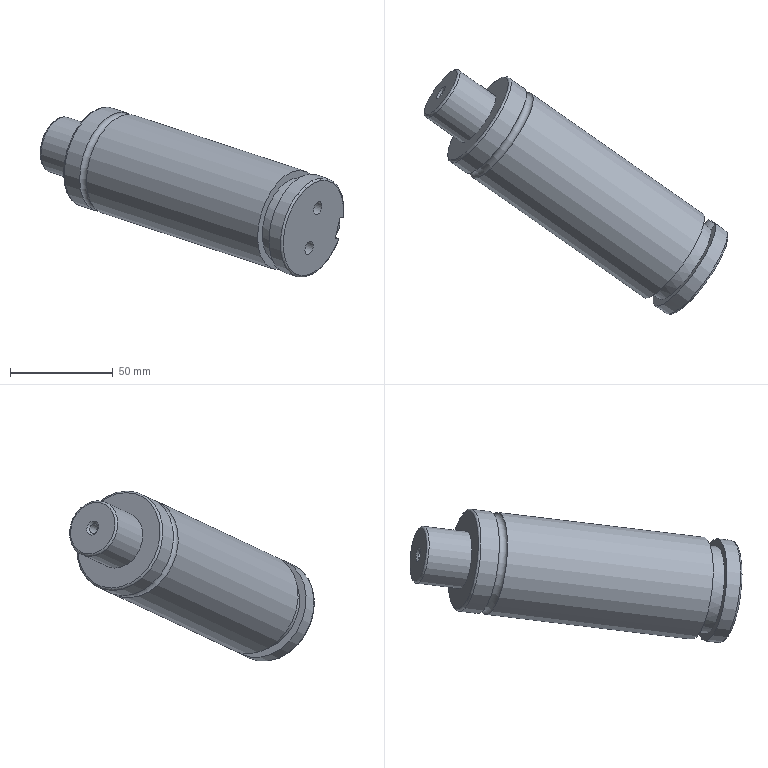Part | NX | features 1 2 | 1 solid | 34 faces | box 148.12 x 119.315 x 82.981 mm | volume 275318 mm3 | plane 16 | cylinder 10 | torus 4 | cone 4 | commonest cylinder face diameters 50.2 x3 6.6 x2 4.9 x1 9.5 x1 11 x1 28 x1
STEP:
#1=CARTESIAN_POINT('',(-931.05,560.37,-211.525));
#2=VERTEX_POINT('',#1);
#3=CARTESIAN_POINT('',(-936.371,564.096,-235.77));
#4=DIRECTION('',(-0.7912,0.554,0.2588));
#5=DIRECTION('',(0.212,-0.1485,0.9659));
#6=AXIS2_PLACEMENT_3D('',#3,#4,#5);
#7=CIRCLE('',#6,25.1);
#8=EDGE_CURVE('',#2,#2,#7,.T.);
#9=ORIENTED_EDGE('',*,*,#8,.T.);
#10=EDGE_LOOP('',(#9));
#11=FACE_BOUND('',#10,.T.);
#12=CARTESIAN_POINT('',(-934.373,562.697,-210.438));
#13=VERTEX_POINT('',#12);
#14=CARTESIAN_POINT('',(-939.694,566.423,-234.683));
#15=DIRECTION('',(-0.7912,0.554,0.2588));
#16=DIRECTION('',(0.212,-0.1485,0.9659));
#17=AXIS2_PLACEMENT_3D('',#14,#15,#16);
#18=CIRCLE('',#17,25.1);
#19=EDGE_CURVE('',#13,#13,#18,.T.);
#20=ORIENTED_EDGE('',*,*,#19,.F.);
#21=EDGE_LOOP('',(#20));
#22=FACE_BOUND('',#21,.T.);
#23=CARTESIAN_POINT('',(-938.033,565.259,-235.227));
#24=DIRECTION('',(-0.7912,0.554,0.2588));
#25=DIRECTION('',(-0.5736,-0.8192,0.));
#26=AXIS2_PLACEMENT_3D('',#23,#24,#25);
#27=TOROIDAL_SURFACE('',#26,25.1,2.1);
#28=ADVANCED_FACE('',(#11,#22),#27,.F.);
#29=CARTESIAN_POINT('',(-941.81,567.905,-208.005));
#30=VERTEX_POINT('',#29);
#31=CARTESIAN_POINT('',(-947.132,571.631,-232.25));
#32=DIRECTION('',(-0.7912,0.554,0.2588));
#33=DIRECTION('',(0.212,-0.1485,0.9659));
#34=AXIS2_PLACEMENT_3D('',#31,#32,#33);
#35=CIRCLE('',#34,25.1);
#36=EDGE_CURVE('',#30,#30,#35,.T.);
#37=ORIENTED_EDGE('',*,*,#36,.T.);
#38=EDGE_LOOP('',(#37));
#39=FACE_BOUND('',#38,.T.);
#40=CARTESIAN_POINT('',(-942.814,568.607,-208.713));
#41=VERTEX_POINT('',#40);
#42=CARTESIAN_POINT('',(-947.923,572.185,-231.991));
#43=DIRECTION('',(-0.7912,0.554,0.2588));
#44=DIRECTION('',(0.212,-0.1485,0.9659));
#45=AXIS2_PLACEMENT_3D('',#42,#43,#44);
#46=CIRCLE('',#45,24.1);
#47=EDGE_CURVE('',#41,#41,#46,.T.);
#48=ORIENTED_EDGE('',*,*,#47,.F.);
#49=EDGE_LOOP('',(#48));
#50=FACE_BOUND('',#49,.T.);
#51=CARTESIAN_POINT('',(-947.132,571.631,-232.25));
#52=DIRECTION('',(-0.7912,0.554,0.2588));
#53=DIRECTION('',(-0.5736,-0.8192,0.));
#54=AXIS2_PLACEMENT_3D('',#51,#52,#53);
#55=TOROIDAL_SURFACE('',#54,24.1,1.);
#56=ADVANCED_FACE('',(#39,#50),#55,.T.);
#57=ORIENTED_EDGE('',*,*,#19,.T.);
#58=EDGE_LOOP('',(#57));
#59=FACE_BOUND('',#58,.T.);
#60=ORIENTED_EDGE('',*,*,#36,.F.);
#61=EDGE_LOOP('',(#60));
#62=FACE_BOUND('',#61,.T.);
#63=CARTESIAN_POINT('',(-943.413,569.027,-233.467));
#64=DIRECTION('',(0.7912,-0.554,-0.2588));
#65=DIRECTION('',(0.5736,0.8192,0.));
#66=AXIS2_PLACEMENT_3D('',#63,#64,#65);
#67=CYLINDRICAL_SURFACE('',#66,25.1);
#68=ADVANCED_FACE('',(#59,#62),#67,.T.);
#69=CARTESIAN_POINT('',(-847.653,501.975,-238.805));
#70=VERTEX_POINT('',#69);
#71=CARTESIAN_POINT('',(-852.974,505.701,-263.05));
#72=DIRECTION('',(-0.7912,0.554,0.2588));
#73=DIRECTION('',(0.212,-0.1485,0.9659));
#74=AXIS2_PLACEMENT_3D('',#71,#72,#73);
#75=CIRCLE('',#74,25.1);
#76=EDGE_CURVE('',#70,#70,#75,.T.);
#77=ORIENTED_EDGE('',*,*,#76,.T.);
#78=EDGE_LOOP('',(#77));
#79=FACE_BOUND('',#78,.T.);
#80=ORIENTED_EDGE('',*,*,#8,.F.);
#81=EDGE_LOOP('',(#80));
#82=FACE_BOUND('',#81,.T.);
#83=CARTESIAN_POINT('',(-889.134,531.02,-251.222));
#84=DIRECTION('',(0.7912,-0.554,-0.2588));
#85=DIRECTION('',(0.5736,0.8192,0.));
#86=AXIS2_PLACEMENT_3D('',#83,#84,#85);
#87=CYLINDRICAL_SURFACE('',#86,25.1);
#88=ADVANCED_FACE('',(#79,#82),#87,.T.);
#89=CARTESIAN_POINT('',(-848.459,502.539,-242.475));
#90=VERTEX_POINT('',#89);
#91=CARTESIAN_POINT('',(-852.974,505.701,-263.05));
#92=DIRECTION('',(-0.7912,0.554,0.2588));
#93=DIRECTION('',(0.212,-0.1485,0.9659));
#94=AXIS2_PLACEMENT_3D('',#91,#92,#93);
#95=CIRCLE('',#94,21.3);
#96=EDGE_CURVE('',#90,#90,#95,.T.);
#97=ORIENTED_EDGE('',*,*,#96,.F.);
#98=EDGE_LOOP('',(#97));
#99=FACE_BOUND('',#98,.T.);
#100=CARTESIAN_POINT('',(-836.663,519.519,-269.81));
#101=VERTEX_POINT('',#100);
#102=CARTESIAN_POINT('',(-834.491,517.998,-259.913));
#103=VERTEX_POINT('',#102);
#104=CARTESIAN_POINT('',(-847.436,501.823,-264.861));
#105=DIRECTION('',(-0.7912,0.554,0.2588));
#106=DIRECTION('',(0.212,-0.1485,0.9659));
#107=AXIS2_PLACEMENT_3D('',#104,#105,#106);
#108=CIRCLE('',#107,21.3);
#109=EDGE_CURVE('',#101,#103,#108,.T.);
#110=ORIENTED_EDGE('',*,*,#109,.T.);
#111=CARTESIAN_POINT('',(-834.491,517.998,-259.913));
#112=CARTESIAN_POINT('',(-835.338,518.713,-260.035));
#113=CARTESIAN_POINT('',(-836.848,520.175,-260.94));
#114=CARTESIAN_POINT('',(-838.206,521.481,-263.862));
#115=CARTESIAN_POINT('',(-838.253,521.159,-267.327));
#116=CARTESIAN_POINT('',(-837.339,520.114,-269.153));
#117=CARTESIAN_POINT('',(-836.663,519.519,-269.81));
#118=B_SPLINE_CURVE_WITH_KNOTS('',3,(#111,#112,#113,#114,#115,#116,#117),.UNSPECIFIED.,.F.,.F.,(4,1,1,1,4),(0.,0.003296,0.006593,0.009889,0.01319),.UNSPECIFIED.);
#119=EDGE_CURVE('',#103,#101,#118,.T.);
#120=ORIENTED_EDGE('',*,*,#119,.T.);
#121=EDGE_LOOP('',(#110,#120));
#122=FACE_BOUND('',#121,.T.);
#123=CARTESIAN_POINT('',(-850.205,503.762,-263.956));
#124=DIRECTION('',(0.7912,-0.554,-0.2588));
#125=DIRECTION('',(0.5736,0.8192,0.));
#126=AXIS2_PLACEMENT_3D('',#123,#124,#125);
#127=CYLINDRICAL_SURFACE('',#126,21.3);
#128=ADVANCED_FACE('',(#99,#122),#127,.T.);
#129=CARTESIAN_POINT('',(-962.362,582.295,-212.774));
#130=VERTEX_POINT('',#129);
#131=CARTESIAN_POINT('',(-965.331,584.374,-226.297));
#132=DIRECTION('',(-0.7912,0.554,0.2588));
#133=DIRECTION('',(0.212,-0.1485,0.9659));
#134=AXIS2_PLACEMENT_3D('',#131,#132,#133);
#135=CIRCLE('',#134,14.);
#136=EDGE_CURVE('',#130,#130,#135,.T.);
#137=ORIENTED_EDGE('',*,*,#136,.T.);
#138=EDGE_LOOP('',(#137));
#139=FACE_BOUND('',#138,.T.);
#140=CARTESIAN_POINT('',(-963.366,582.998,-213.482));
#141=VERTEX_POINT('',#140);
#142=CARTESIAN_POINT('',(-966.122,584.928,-226.039));
#143=DIRECTION('',(-0.7912,0.554,0.2588));
#144=DIRECTION('',(0.212,-0.1485,0.9659));
#145=AXIS2_PLACEMENT_3D('',#142,#143,#144);
#146=CIRCLE('',#145,13.);
#147=EDGE_CURVE('',#141,#141,#146,.T.);
#148=ORIENTED_EDGE('',*,*,#147,.F.);
#149=EDGE_LOOP('',(#148));
#150=FACE_BOUND('',#149,.T.);
#151=CARTESIAN_POINT('',(-965.331,584.374,-226.297));
#152=DIRECTION('',(-0.7912,0.554,0.2588));
#153=DIRECTION('',(-0.5736,-0.8192,0.));
#154=AXIS2_PLACEMENT_3D('',#151,#152,#153);
#155=TOROIDAL_SURFACE('',#154,13.,1.);
#156=ADVANCED_FACE('',(#139,#150),#155,.T.);
#157=CARTESIAN_POINT('',(-944.955,570.107,-218.468));
#158=VERTEX_POINT('',#157);
#159=CARTESIAN_POINT('',(-947.923,572.185,-231.991));
#160=DIRECTION('',(0.7912,-0.554,-0.2588));
#161=DIRECTION('',(0.212,-0.1485,0.9659));
#162=AXIS2_PLACEMENT_3D('',#159,#160,#161);
#163=CIRCLE('',#162,14.);
#164=EDGE_CURVE('',#158,#158,#163,.T.);
#165=ORIENTED_EDGE('',*,*,#164,.F.);
#166=EDGE_LOOP('',(#165));
#167=FACE_BOUND('',#166,.T.);
#168=ORIENTED_EDGE('',*,*,#136,.F.);
#169=EDGE_LOOP('',(#168));
#170=FACE_BOUND('',#169,.T.);
#171=CARTESIAN_POINT('',(-956.627,578.279,-229.144));
#172=DIRECTION('',(0.7912,-0.554,-0.2588));
#173=DIRECTION('',(0.5736,0.8192,0.));
#174=AXIS2_PLACEMENT_3D('',#171,#172,#173);
#175=CYLINDRICAL_SURFACE('',#174,14.);
#176=ADVANCED_FACE('',(#167,#170),#175,.T.);
#177=CARTESIAN_POINT('',(-839.685,496.396,-260.46));
#178=VERTEX_POINT('',#177);
#179=CARTESIAN_POINT('',(-838.986,495.906,-257.273));
#180=DIRECTION('',(-0.7912,0.554,0.2588));
#181=DIRECTION('',(-0.212,0.1485,-0.9659));
#182=AXIS2_PLACEMENT_3D('',#179,#180,#181);
#183=CIRCLE('',#182,3.3);
#184=EDGE_CURVE('',#178,#178,#183,.T.);
#185=ORIENTED_EDGE('',*,*,#184,.F.);
#186=EDGE_LOOP('',(#185));
#187=FACE_BOUND('',#186,.T.);
#188=CARTESIAN_POINT('',(-848.547,502.601,-257.561));
#189=VERTEX_POINT('',#188);
#190=CARTESIAN_POINT('',(-847.848,502.111,-254.374));
#191=DIRECTION('',(0.7912,-0.554,-0.2588));
#192=DIRECTION('',(-0.212,0.1485,-0.9659));
#193=AXIS2_PLACEMENT_3D('',#190,#191,#192);
#194=CIRCLE('',#193,3.3);
#195=EDGE_CURVE('',#189,#189,#194,.T.);
#196=ORIENTED_EDGE('',*,*,#195,.F.);
#197=EDGE_LOOP('',(#196));
#198=FACE_BOUND('',#197,.T.);
#199=CARTESIAN_POINT('',(-843.417,499.009,-255.823));
#200=DIRECTION('',(-0.7912,0.554,0.2588));
#201=DIRECTION('',(-0.5736,-0.8192,0.));
#202=AXIS2_PLACEMENT_3D('',#199,#200,#201);
#203=CYLINDRICAL_SURFACE('',#202,3.3);
#204=ADVANCED_FACE('',(#187,#198),#203,.F.);
#205=ORIENTED_EDGE('',*,*,#195,.T.);
#206=EDGE_LOOP('',(#205));
#207=FACE_BOUND('',#206,.T.);
#208=CARTESIAN_POINT('',(-845.711,500.615,-255.073));
#209=VERTEX_POINT('',#208);
#210=VERTEX_LOOP('',#209);
#211=FACE_BOUND('',#210,.T.);
#212=CARTESIAN_POINT('',(-846.779,501.363,-254.723));
#213=DIRECTION('',(-0.7912,0.554,0.2588));
#214=DIRECTION('',(-0.5736,-0.8192,0.));
#215=AXIS2_PLACEMENT_3D('',#212,#213,#214);
#216=CONICAL_SURFACE('',#215,1.65,0.8851);
#217=ADVANCED_FACE('',(#207,#211),#216,.T.);
#218=CARTESIAN_POINT('',(-965.38,584.408,-222.658));
#219=VERTEX_POINT('',#218);
#220=CARTESIAN_POINT('',(-966.122,584.928,-226.039));
#221=DIRECTION('',(0.7912,-0.554,-0.2588));
#222=DIRECTION('',(0.212,-0.1485,0.9659));
#223=AXIS2_PLACEMENT_3D('',#220,#221,#222);
#224=CIRCLE('',#223,3.5);
#225=EDGE_CURVE('',#219,#219,#224,.T.);
#226=ORIENTED_EDGE('',*,*,#225,.F.);
#227=EDGE_LOOP('',(#226));
#228=FACE_BOUND('',#227,.T.);
#229=CARTESIAN_POINT('',(-964.772,583.982,-223.944));
#230=VERTEX_POINT('',#229);
#231=CARTESIAN_POINT('',(-965.291,584.346,-226.31));
#232=DIRECTION('',(-0.7912,0.554,0.2588));
#233=DIRECTION('',(0.212,-0.1485,0.9659));
#234=AXIS2_PLACEMENT_3D('',#231,#232,#233);
#235=CIRCLE('',#234,2.45);
#236=EDGE_CURVE('',#230,#230,#235,.T.);
#237=ORIENTED_EDGE('',*,*,#236,.F.);
#238=EDGE_LOOP('',(#237));
#239=FACE_BOUND('',#238,.T.);
#240=CARTESIAN_POINT('',(-965.706,584.637,-226.174));
#241=DIRECTION('',(-0.7912,0.554,0.2588));
#242=DIRECTION('',(-0.5736,-0.8192,0.));
#243=AXIS2_PLACEMENT_3D('',#240,#241,#242);
#244=CONICAL_SURFACE('',#243,2.975,0.7854);
#245=ADVANCED_FACE('',(#228,#239),#244,.F.);
#246=ORIENTED_EDGE('',*,*,#236,.T.);
#247=EDGE_LOOP('',(#246));
#248=FACE_BOUND('',#247,.T.);
#249=CARTESIAN_POINT('',(-960.459,580.963,-225.354));
#250=VERTEX_POINT('',#249);
#251=CARTESIAN_POINT('',(-960.979,581.326,-227.721));
#252=DIRECTION('',(-0.7912,0.554,0.2588));
#253=DIRECTION('',(0.212,-0.1485,0.9659));
#254=AXIS2_PLACEMENT_3D('',#251,#252,#253);
#255=CIRCLE('',#254,2.45);
#256=EDGE_CURVE('',#250,#250,#255,.T.);
#257=ORIENTED_EDGE('',*,*,#256,.F.);
#258=EDGE_LOOP('',(#257));
#259=FACE_BOUND('',#258,.T.);
#260=CARTESIAN_POINT('',(-963.135,582.836,-227.016));
#261=DIRECTION('',(0.7912,-0.554,-0.2588));
#262=DIRECTION('',(0.5736,0.8192,0.));
#263=AXIS2_PLACEMENT_3D('',#260,#261,#262);
#264=CYLINDRICAL_SURFACE('',#263,2.45);
#265=ADVANCED_FACE('',(#248,#259),#264,.F.);
#266=CARTESIAN_POINT('',(-960.187,580.772,-227.98));
#267=VERTEX_POINT('',#266);
#268=VERTEX_LOOP('',#267);
#269=FACE_BOUND('',#268,.T.);
#270=ORIENTED_EDGE('',*,*,#256,.T.);
#271=EDGE_LOOP('',(#270));
#272=FACE_BOUND('',#271,.T.);
#273=CARTESIAN_POINT('',(-960.583,581.049,-227.85));
#274=DIRECTION('',(-0.7912,0.554,0.2588));
#275=DIRECTION('',(-0.5736,-0.8192,0.));
#276=AXIS2_PLACEMENT_3D('',#273,#274,#275);
#277=CONICAL_SURFACE('',#276,1.225,1.183);
#278=ADVANCED_FACE('',(#269,#272),#277,.F.);
#279=CARTESIAN_POINT('',(-849.951,503.584,-274.391));
#280=VERTEX_POINT('',#279);
#281=VERTEX_LOOP('',#280);
#282=FACE_BOUND('',#281,.T.);
#283=CARTESIAN_POINT('',(-851.388,504.59,-270.505));
#284=VERTEX_POINT('',#283);
#285=CARTESIAN_POINT('',(-852.088,505.08,-273.692));
#286=DIRECTION('',(-0.7912,0.554,0.2588));
#287=DIRECTION('',(0.212,-0.1485,0.9659));
#288=AXIS2_PLACEMENT_3D('',#285,#286,#287);
#289=CIRCLE('',#288,3.3);
#290=EDGE_CURVE('',#284,#284,#289,.T.);
#291=ORIENTED_EDGE('',*,*,#290,.F.);
#292=EDGE_LOOP('',(#291));
#293=FACE_BOUND('',#292,.T.);
#294=CARTESIAN_POINT('',(-851.02,504.332,-274.042));
#295=DIRECTION('',(-0.7912,0.554,0.2588));
#296=DIRECTION('',(-0.5736,-0.8192,0.));
#297=AXIS2_PLACEMENT_3D('',#294,#295,#296);
#298=CONICAL_SURFACE('',#297,1.65,0.8851);
#299=ADVANCED_FACE('',(#282,#293),#298,.T.);
#300=ORIENTED_EDGE('',*,*,#290,.T.);
#301=EDGE_LOOP('',(#300));
#302=FACE_BOUND('',#301,.T.);
#303=CARTESIAN_POINT('',(-842.526,498.385,-273.404));
#304=VERTEX_POINT('',#303);
#305=CARTESIAN_POINT('',(-843.226,498.875,-276.591));
#306=DIRECTION('',(-0.7912,0.554,0.2588));
#307=DIRECTION('',(0.212,-0.1485,0.9659));
#308=AXIS2_PLACEMENT_3D('',#305,#306,#307);
#309=CIRCLE('',#308,3.3);
#310=EDGE_CURVE('',#304,#304,#309,.T.);
#311=ORIENTED_EDGE('',*,*,#310,.F.);
#312=EDGE_LOOP('',(#311));
#313=FACE_BOUND('',#312,.T.);
#314=CARTESIAN_POINT('',(-847.657,501.978,-275.142));
#315=DIRECTION('',(0.7912,-0.554,-0.2588));
#316=DIRECTION('',(0.5736,0.8192,0.));
#317=AXIS2_PLACEMENT_3D('',#314,#315,#316);
#318=CYLINDRICAL_SURFACE('',#317,3.3);
#319=ADVANCED_FACE('',(#302,#313),#318,.F.);
#320=CARTESIAN_POINT('',(-829.016,518.822,-271.986));
#321=VERTEX_POINT('',#320);
#322=CARTESIAN_POINT('',(-826.684,517.189,-261.361));
#323=VERTEX_POINT('',#322);
#324=CARTESIAN_POINT('',(-841.897,497.945,-266.673));
#325=DIRECTION('',(-0.7912,0.554,0.2588));
#326=DIRECTION('',(0.212,-0.1485,0.9659));
#327=AXIS2_PLACEMENT_3D('',#324,#325,#326);
#328=CIRCLE('',#327,25.1);
#329=EDGE_CURVE('',#321,#323,#328,.T.);
#330=ORIENTED_EDGE('',*,*,#329,.T.);
#331=CARTESIAN_POINT('',(-830.64,519.959,-260.066));
#332=VERTEX_POINT('',#331);
#333=CARTESIAN_POINT('',(-828.662,518.574,-260.714));
#334=DIRECTION('',(-0.7912,0.554,0.2588));
#335=VECTOR('',#334,1000.);
#336=LINE('',#333,#335);
#337=EDGE_CURVE('',#323,#332,#336,.T.);
#338=ORIENTED_EDGE('',*,*,#337,.T.);
#339=CARTESIAN_POINT('',(-832.256,521.19,-259.913));
#340=VERTEX_POINT('',#339);
#341=CARTESIAN_POINT('',(-830.64,519.959,-260.066));
#342=CARTESIAN_POINT('',(-831.187,520.342,-259.888));
#343=CARTESIAN_POINT('',(-831.725,520.754,-259.837));
#344=CARTESIAN_POINT('',(-832.256,521.19,-259.913));
#345=B_SPLINE_CURVE_WITH_KNOTS('',3,(#341,#342,#343,#344),.UNSPECIFIED.,.F.,.F.,(4,4),(0.,0.002037),.UNSPECIFIED.);
#346=EDGE_CURVE('',#332,#340,#345,.T.);
#347=ORIENTED_EDGE('',*,*,#346,.T.);
#348=CARTESIAN_POINT('',(-834.428,522.711,-269.81));
#349=VERTEX_POINT('',#348);
#350=CARTESIAN_POINT('',(-847.436,501.823,-264.861));
#351=DIRECTION('',(0.7912,-0.554,-0.2588));
#352=DIRECTION('',(0.212,-0.1485,0.9659));
#353=AXIS2_PLACEMENT_3D('',#350,#351,#352);
#354=CIRCLE('',#353,25.1);
#355=EDGE_CURVE('',#340,#349,#354,.T.);
#356=ORIENTED_EDGE('',*,*,#355,.T.);
#357=CARTESIAN_POINT('',(-832.972,521.592,-270.692));
#358=VERTEX_POINT('',#357);
#359=CARTESIAN_POINT('',(-834.428,522.711,-269.81));
#360=CARTESIAN_POINT('',(-834.003,522.35,-270.219));
#361=CARTESIAN_POINT('',(-833.519,521.975,-270.513));
#362=CARTESIAN_POINT('',(-832.972,521.592,-270.692));
#363=B_SPLINE_CURVE_WITH_KNOTS('',3,(#359,#360,#361,#362),.UNSPECIFIED.,.F.,.F.,(4,4),(0.,0.002037),.UNSPECIFIED.);
#364=EDGE_CURVE('',#349,#358,#363,.T.);
#365=ORIENTED_EDGE('',*,*,#364,.T.);
#366=CARTESIAN_POINT('',(-830.994,520.207,-271.339));
#367=DIRECTION('',(0.7912,-0.554,-0.2588));
#368=VECTOR('',#367,1000.);
#369=LINE('',#366,#368);
#370=EDGE_CURVE('',#358,#321,#369,.T.);
#371=ORIENTED_EDGE('',*,*,#370,.T.);
#372=EDGE_LOOP('',(#330,#338,#347,#356,#365,#371));
#373=FACE_BOUND('',#372,.T.);
#374=CARTESIAN_POINT('',(-889.134,531.02,-251.222));
#375=DIRECTION('',(0.7912,-0.554,-0.2588));
#376=DIRECTION('',(0.5736,0.8192,0.));
#377=AXIS2_PLACEMENT_3D('',#374,#375,#376);
#378=CYLINDRICAL_SURFACE('',#377,25.1);
#379=ADVANCED_FACE('',(#373),#378,.T.);
#380=CARTESIAN_POINT('',(-826.481,515.795,-261.619));
#381=VERTEX_POINT('',#380);
#382=CARTESIAN_POINT('',(-826.481,515.795,-261.619));
#383=CARTESIAN_POINT('',(-826.174,516.233,-261.619));
#384=CARTESIAN_POINT('',(-826.26,516.892,-261.499));
#385=CARTESIAN_POINT('',(-826.684,517.189,-261.361));
#386=B_SPLINE_CURVE_WITH_KNOTS('',3,(#382,#383,#384,#385),.UNSPECIFIED.,.F.,.F.,(4,4),(0.,0.001583),.UNSPECIFIED.);
#387=EDGE_CURVE('',#381,#323,#386,.T.);
#388=ORIENTED_EDGE('',*,*,#387,.T.);
#389=ORIENTED_EDGE('',*,*,#329,.F.);
#390=CARTESIAN_POINT('',(-828.813,517.428,-272.245));
#391=VERTEX_POINT('',#390);
#392=CARTESIAN_POINT('',(-829.016,518.822,-271.986));
#393=CARTESIAN_POINT('',(-828.593,518.526,-272.124));
#394=CARTESIAN_POINT('',(-828.507,517.866,-272.245));
#395=CARTESIAN_POINT('',(-828.813,517.428,-272.245));
#396=B_SPLINE_CURVE_WITH_KNOTS('',3,(#392,#393,#394,#395),.UNSPECIFIED.,.F.,.F.,(4,4),(0.,0.001583),.UNSPECIFIED.);
#397=EDGE_CURVE('',#321,#391,#396,.T.);
#398=ORIENTED_EDGE('',*,*,#397,.T.);
#399=CARTESIAN_POINT('',(-841.106,497.391,-266.932));
#400=DIRECTION('',(-0.7912,0.554,0.2588));
#401=DIRECTION('',(0.212,-0.1485,0.9659));
#402=AXIS2_PLACEMENT_3D('',#399,#400,#401);
#403=CIRCLE('',#402,24.1);
#404=EDGE_CURVE('',#391,#381,#403,.T.);
#405=ORIENTED_EDGE('',*,*,#404,.T.);
#406=EDGE_LOOP('',(#388,#389,#398,#405));
#407=FACE_BOUND('',#406,.T.);
#408=CARTESIAN_POINT('',(-841.897,497.945,-266.673));
#409=DIRECTION('',(-0.7912,0.554,0.2588));
#410=DIRECTION('',(-0.5736,-0.8192,0.));
#411=AXIS2_PLACEMENT_3D('',#408,#409,#410);
#412=TOROIDAL_SURFACE('',#411,24.1,1.);
#413=ADVANCED_FACE('',(#407),#412,.T.);
#414=CARTESIAN_POINT('',(-833.031,516.884,-260.791));
#415=VERTEX_POINT('',#414);
#416=CARTESIAN_POINT('',(-834.038,517.589,-265.379));
#417=DIRECTION('',(-0.5736,-0.8192,0.));
#418=DIRECTION('',(0.212,-0.1485,0.9659));
#419=AXIS2_PLACEMENT_3D('',#416,#417,#418);
#420=CIRCLE('',#419,4.75);
#421=EDGE_CURVE('',#415,#415,#420,.T.);
#422=ORIENTED_EDGE('',*,*,#421,.F.);
#423=EDGE_LOOP('',(#422));
#424=FACE_BOUND('',#423,.T.);
#425=CARTESIAN_POINT('',(-831.023,519.751,-260.791));
#426=VERTEX_POINT('',#425);
#427=CARTESIAN_POINT('',(-832.03,520.456,-265.379));
#428=DIRECTION('',(-0.5736,-0.8192,0.));
#429=DIRECTION('',(0.212,-0.1485,0.9659));
#430=AXIS2_PLACEMENT_3D('',#427,#428,#429);
#431=CIRCLE('',#430,4.75);
#432=EDGE_CURVE('',#426,#426,#431,.T.);
#433=ORIENTED_EDGE('',*,*,#432,.T.);
#434=EDGE_LOOP('',(#433));
#435=FACE_BOUND('',#434,.T.);
#436=CARTESIAN_POINT('',(-845.853,500.715,-265.379));
#437=DIRECTION('',(-0.5736,-0.8192,0.));
#438=DIRECTION('',(0.212,-0.1485,0.9659));
#439=AXIS2_PLACEMENT_3D('',#436,#437,#438);
#440=CYLINDRICAL_SURFACE('',#439,4.75);
#441=ADVANCED_FACE('',(#424,#435),#440,.T.);
#442=CARTESIAN_POINT('',(-833.895,515.658,-264.154));
#443=VERTEX_POINT('',#442);
#444=CARTESIAN_POINT('',(-833.527,515.401,-265.827));
#445=VERTEX_POINT('',#444);
#446=CARTESIAN_POINT('',(-833.895,515.658,-264.154));
#447=DIRECTION('',(0.212,-0.1485,-0.9659));
#448=VECTOR('',#447,1000.);
#449=LINE('',#446,#448);
#450=EDGE_CURVE('',#443,#445,#449,.T.);
#451=ORIENTED_EDGE('',*,*,#450,.F.);
#452=CARTESIAN_POINT('',(-831.027,519.754,-264.154));
#453=VERTEX_POINT('',#452);
#454=CARTESIAN_POINT('',(-831.027,519.754,-264.154));
#455=DIRECTION('',(-0.5736,-0.8192,0.));
#456=VECTOR('',#455,1000.);
#457=LINE('',#454,#456);
#458=EDGE_CURVE('',#453,#443,#457,.T.);
#459=ORIENTED_EDGE('',*,*,#458,.F.);
#460=CARTESIAN_POINT('',(-830.66,519.497,-265.827));
#461=VERTEX_POINT('',#460);
#462=CARTESIAN_POINT('',(-830.617,519.467,-266.021));
#463=DIRECTION('',(-0.212,0.1485,0.9659));
#464=VECTOR('',#463,1000.);
#465=LINE('',#462,#464);
#466=EDGE_CURVE('',#461,#453,#465,.T.);
#467=ORIENTED_EDGE('',*,*,#466,.F.);
#468=CARTESIAN_POINT('',(-830.66,519.497,-265.827));
#469=DIRECTION('',(-0.5736,-0.8192,0.));
#470=VECTOR('',#469,1000.);
#471=LINE('',#468,#470);
#472=EDGE_CURVE('',#461,#445,#471,.T.);
#473=ORIENTED_EDGE('',*,*,#472,.T.);
#474=EDGE_LOOP('',(#451,#459,#467,#473));
#475=FACE_BOUND('',#474,.T.);
#476=CARTESIAN_POINT('',(-831.027,519.754,-264.154));
#477=DIRECTION('',(0.7912,-0.554,0.2588));
#478=DIRECTION('',(-0.212,0.1485,0.9659));
#479=AXIS2_PLACEMENT_3D('',#476,#477,#478);
#480=PLANE('',#479);
#481=ADVANCED_FACE('',(#475),#480,.F.);
#482=CARTESIAN_POINT('',(-834.531,516.103,-267.052));
#483=VERTEX_POINT('',#482);
#484=CARTESIAN_POINT('',(-833.527,515.401,-265.827));
#485=DIRECTION('',(-0.5792,0.4056,-0.7071));
#486=VECTOR('',#485,1000.);
#487=LINE('',#484,#486);
#488=EDGE_CURVE('',#445,#483,#487,.T.);
#489=ORIENTED_EDGE('',*,*,#488,.F.);
#490=ORIENTED_EDGE('',*,*,#472,.F.);
#491=CARTESIAN_POINT('',(-831.663,520.199,-267.052));
#492=VERTEX_POINT('',#491);
#493=CARTESIAN_POINT('',(-830.042,519.064,-265.073));
#494=DIRECTION('',(0.5792,-0.4056,0.7071));
#495=VECTOR('',#494,1000.);
#496=LINE('',#493,#495);
#497=EDGE_CURVE('',#492,#461,#496,.T.);
#498=ORIENTED_EDGE('',*,*,#497,.F.);
#499=CARTESIAN_POINT('',(-831.663,520.199,-267.052));
#500=DIRECTION('',(-0.5736,-0.8192,0.));
#501=VECTOR('',#500,1000.);
#502=LINE('',#499,#501);
#503=EDGE_CURVE('',#492,#483,#502,.T.);
#504=ORIENTED_EDGE('',*,*,#503,.T.);
#505=EDGE_LOOP('',(#489,#490,#498,#504));
#506=FACE_BOUND('',#505,.T.);
#507=CARTESIAN_POINT('',(-830.66,519.497,-265.827));
#508=DIRECTION('',(0.5792,-0.4056,-0.7071));
#509=DIRECTION('',(0.5792,-0.4056,0.7071));
#510=AXIS2_PLACEMENT_3D('',#507,#508,#509);
#511=PLANE('',#510);
#512=ADVANCED_FACE('',(#506),#511,.F.);
#513=CARTESIAN_POINT('',(-835.901,517.063,-266.604));
#514=VERTEX_POINT('',#513);
#515=CARTESIAN_POINT('',(-834.531,516.103,-267.052));
#516=DIRECTION('',(-0.7912,0.554,0.2588));
#517=VECTOR('',#516,1000.);
#518=LINE('',#515,#517);
#519=EDGE_CURVE('',#483,#514,#518,.T.);
#520=ORIENTED_EDGE('',*,*,#519,.F.);
#521=ORIENTED_EDGE('',*,*,#503,.F.);
#522=CARTESIAN_POINT('',(-833.033,521.159,-266.604));
#523=VERTEX_POINT('',#522);
#524=CARTESIAN_POINT('',(-829.632,518.777,-267.716));
#525=DIRECTION('',(0.7912,-0.554,-0.2588));
#526=VECTOR('',#525,1000.);
#527=LINE('',#524,#526);
#528=EDGE_CURVE('',#523,#492,#527,.T.);
#529=ORIENTED_EDGE('',*,*,#528,.F.);
#530=CARTESIAN_POINT('',(-833.033,521.159,-266.604));
#531=DIRECTION('',(-0.5736,-0.8192,0.));
#532=VECTOR('',#531,1000.);
#533=LINE('',#530,#532);
#534=EDGE_CURVE('',#523,#514,#533,.T.);
#535=ORIENTED_EDGE('',*,*,#534,.T.);
#536=EDGE_LOOP('',(#520,#521,#529,#535));
#537=FACE_BOUND('',#536,.T.);
#538=CARTESIAN_POINT('',(-831.663,520.199,-267.052));
#539=DIRECTION('',(-0.212,0.1485,-0.9659));
#540=DIRECTION('',(-0.5736,-0.8192,0.));
#541=AXIS2_PLACEMENT_3D('',#538,#539,#540);
#542=PLANE('',#541);
#543=ADVANCED_FACE('',(#537),#542,.F.);
#544=CARTESIAN_POINT('',(-836.268,517.32,-264.931));
#545=VERTEX_POINT('',#544);
#546=CARTESIAN_POINT('',(-835.901,517.063,-266.604));
#547=DIRECTION('',(-0.212,0.1485,0.9659));
#548=VECTOR('',#547,1000.);
#549=LINE('',#546,#548);
#550=EDGE_CURVE('',#514,#545,#549,.T.);
#551=ORIENTED_EDGE('',*,*,#550,.F.);
#552=ORIENTED_EDGE('',*,*,#534,.F.);
#553=CARTESIAN_POINT('',(-833.401,521.416,-264.931));
#554=VERTEX_POINT('',#553);
#555=CARTESIAN_POINT('',(-832.807,521.,-267.634));
#556=DIRECTION('',(0.212,-0.1485,-0.9659));
#557=VECTOR('',#556,1000.);
#558=LINE('',#555,#557);
#559=EDGE_CURVE('',#554,#523,#558,.T.);
#560=ORIENTED_EDGE('',*,*,#559,.F.);
#561=CARTESIAN_POINT('',(-833.401,521.416,-264.931));
#562=DIRECTION('',(-0.5736,-0.8192,0.));
#563=VECTOR('',#562,1000.);
#564=LINE('',#561,#563);
#565=EDGE_CURVE('',#554,#545,#564,.T.);
#566=ORIENTED_EDGE('',*,*,#565,.T.);
#567=EDGE_LOOP('',(#551,#552,#560,#566));
#568=FACE_BOUND('',#567,.T.);
#569=CARTESIAN_POINT('',(-833.033,521.159,-266.604));
#570=DIRECTION('',(-0.7912,0.554,-0.2588));
#571=DIRECTION('',(0.212,-0.1485,-0.9659));
#572=AXIS2_PLACEMENT_3D('',#569,#570,#571);
#573=PLANE('',#572);
#574=ADVANCED_FACE('',(#568),#573,.F.);
#575=CARTESIAN_POINT('',(-835.265,516.618,-263.706));
#576=VERTEX_POINT('',#575);
#577=CARTESIAN_POINT('',(-836.268,517.32,-264.931));
#578=DIRECTION('',(0.5792,-0.4056,0.7071));
#579=VECTOR('',#578,1000.);
#580=LINE('',#577,#579);
#581=EDGE_CURVE('',#545,#576,#580,.T.);
#582=ORIENTED_EDGE('',*,*,#581,.F.);
#583=ORIENTED_EDGE('',*,*,#565,.F.);
#584=CARTESIAN_POINT('',(-832.397,520.713,-263.706));
#585=VERTEX_POINT('',#584);
#586=CARTESIAN_POINT('',(-832.281,520.632,-263.564));
#587=DIRECTION('',(-0.5792,0.4056,-0.7071));
#588=VECTOR('',#587,1000.);
#589=LINE('',#586,#588);
#590=EDGE_CURVE('',#585,#554,#589,.T.);
#591=ORIENTED_EDGE('',*,*,#590,.F.);
#592=CARTESIAN_POINT('',(-832.397,520.713,-263.706));
#593=DIRECTION('',(-0.5736,-0.8192,0.));
#594=VECTOR('',#593,1000.);
#595=LINE('',#592,#594);
#596=EDGE_CURVE('',#585,#576,#595,.T.);
#597=ORIENTED_EDGE('',*,*,#596,.T.);
#598=EDGE_LOOP('',(#582,#583,#591,#597));
#599=FACE_BOUND('',#598,.T.);
#600=CARTESIAN_POINT('',(-833.401,521.416,-264.931));
#601=DIRECTION('',(-0.5792,0.4056,0.7071));
#602=DIRECTION('',(-0.5792,0.4056,-0.7071));
#603=AXIS2_PLACEMENT_3D('',#600,#601,#602);
#604=PLANE('',#603);
#605=ADVANCED_FACE('',(#599),#604,.F.);
#606=CARTESIAN_POINT('',(-835.265,516.618,-263.706));
#607=DIRECTION('',(0.7912,-0.554,-0.2588));
#608=VECTOR('',#607,1000.);
#609=LINE('',#606,#608);
#610=EDGE_CURVE('',#576,#443,#609,.T.);
#611=ORIENTED_EDGE('',*,*,#610,.F.);
#612=ORIENTED_EDGE('',*,*,#596,.F.);
#613=CARTESIAN_POINT('',(-829.681,518.811,-264.595));
#614=DIRECTION('',(-0.7912,0.554,0.2588));
#615=VECTOR('',#614,1000.);
#616=LINE('',#613,#615);
#617=EDGE_CURVE('',#453,#585,#616,.T.);
#618=ORIENTED_EDGE('',*,*,#617,.F.);
#619=ORIENTED_EDGE('',*,*,#458,.T.);
#620=EDGE_LOOP('',(#611,#612,#618,#619));
#621=FACE_BOUND('',#620,.T.);
#622=CARTESIAN_POINT('',(-832.397,520.713,-263.706));
#623=DIRECTION('',(0.212,-0.1485,0.9659));
#624=DIRECTION('',(0.5736,0.8192,0.));
#625=AXIS2_PLACEMENT_3D('',#622,#623,#624);
#626=PLANE('',#625);
#627=ADVANCED_FACE('',(#621),#626,.F.);
#628=ORIENTED_EDGE('',*,*,#450,.T.);
#629=ORIENTED_EDGE('',*,*,#488,.T.);
#630=ORIENTED_EDGE('',*,*,#519,.T.);
#631=ORIENTED_EDGE('',*,*,#550,.T.);
#632=ORIENTED_EDGE('',*,*,#581,.T.);
#633=ORIENTED_EDGE('',*,*,#610,.T.);
#634=EDGE_LOOP('',(#628,#629,#630,#631,#632,#633));
#635=FACE_BOUND('',#634,.T.);
#636=CARTESIAN_POINT('',(-834.898,516.361,-265.379));
#637=DIRECTION('',(0.5736,0.8192,0.));
#638=DIRECTION('',(-0.212,0.1485,-0.9659));
#639=AXIS2_PLACEMENT_3D('',#636,#637,#638);
#640=PLANE('',#639);
#641=ADVANCED_FACE('',(#635),#640,.T.);
#642=ORIENTED_EDGE('',*,*,#466,.T.);
#643=ORIENTED_EDGE('',*,*,#617,.T.);
#644=ORIENTED_EDGE('',*,*,#590,.T.);
#645=ORIENTED_EDGE('',*,*,#559,.T.);
#646=ORIENTED_EDGE('',*,*,#528,.T.);
#647=ORIENTED_EDGE('',*,*,#497,.T.);
#648=EDGE_LOOP('',(#642,#643,#644,#645,#646,#647));
#649=FACE_BOUND('',#648,.T.);
#650=ORIENTED_EDGE('',*,*,#432,.F.);
#651=EDGE_LOOP('',(#650));
#652=FACE_BOUND('',#651,.T.);
#653=CARTESIAN_POINT('',(-827.283,517.132,-266.932));
#654=DIRECTION('',(-0.5736,-0.8192,0.));
#655=DIRECTION('',(0.212,-0.1485,0.9659));
#656=AXIS2_PLACEMENT_3D('',#653,#654,#655);
#657=PLANE('',#656);
#658=ADVANCED_FACE('',(#649,#652),#657,.F.);
#659=ORIENTED_EDGE('',*,*,#370,.F.);
#660=CARTESIAN_POINT('',(-835.204,518.406,-270.692));
#661=VERTEX_POINT('',#660);
#662=CARTESIAN_POINT('',(-832.623,522.092,-270.692));
#663=DIRECTION('',(-0.5736,-0.8192,0.));
#664=VECTOR('',#663,1000.);
#665=LINE('',#662,#664);
#666=EDGE_CURVE('',#358,#661,#665,.T.);
#667=ORIENTED_EDGE('',*,*,#666,.T.);
#668=CARTESIAN_POINT('',(-830.456,515.082,-272.245));
#669=VERTEX_POINT('',#668);
#670=CARTESIAN_POINT('',(-835.204,518.406,-270.692));
#671=DIRECTION('',(-0.7912,0.554,0.2588));
#672=VECTOR('',#671,1000.);
#673=LINE('',#670,#672);
#674=EDGE_CURVE('',#669,#661,#673,.T.);
#675=ORIENTED_EDGE('',*,*,#674,.F.);
#676=CARTESIAN_POINT('',(-835.073,508.487,-272.245));
#677=DIRECTION('',(-0.5736,-0.8192,0.));
#678=VECTOR('',#677,1000.);
#679=LINE('',#676,#678);
#680=EDGE_CURVE('',#391,#669,#679,.T.);
#681=ORIENTED_EDGE('',*,*,#680,.F.);
#682=ORIENTED_EDGE('',*,*,#397,.F.);
#683=EDGE_LOOP('',(#659,#667,#675,#681,#682));
#684=FACE_BOUND('',#683,.T.);
#685=CARTESIAN_POINT('',(-827.875,518.768,-272.245));
#686=DIRECTION('',(-0.212,0.1485,-0.9659));
#687=DIRECTION('',(-0.5736,-0.8192,0.));
#688=AXIS2_PLACEMENT_3D('',#685,#686,#687);
#689=PLANE('',#688);
#690=ADVANCED_FACE('',(#684),#689,.F.);
#691=ORIENTED_EDGE('',*,*,#364,.F.);
#692=CARTESIAN_POINT('',(-835.416,521.301,-269.81));
#693=DIRECTION('',(0.5736,0.8192,0.));
#694=VECTOR('',#693,1000.);
#695=LINE('',#692,#694);
#696=EDGE_CURVE('',#101,#349,#695,.T.);
#697=ORIENTED_EDGE('',*,*,#696,.F.);
#698=ORIENTED_EDGE('',*,*,#119,.F.);
#699=CARTESIAN_POINT('',(-833.243,519.78,-259.913));
#700=DIRECTION('',(-0.5736,-0.8192,0.));
#701=VECTOR('',#700,1000.);
#702=LINE('',#699,#701);
#703=EDGE_CURVE('',#340,#103,#702,.T.);
#704=ORIENTED_EDGE('',*,*,#703,.F.);
#705=ORIENTED_EDGE('',*,*,#346,.F.);
#706=CARTESIAN_POINT('',(-832.872,516.773,-260.066));
#707=VERTEX_POINT('',#706);
#708=CARTESIAN_POINT('',(-830.29,520.459,-260.066));
#709=DIRECTION('',(-0.5736,-0.8192,0.));
#710=VECTOR('',#709,1000.);
#711=LINE('',#708,#710);
#712=EDGE_CURVE('',#332,#707,#711,.T.);
#713=ORIENTED_EDGE('',*,*,#712,.T.);
#714=CARTESIAN_POINT('',(-834.038,517.589,-265.379));
#715=DIRECTION('',(0.5736,0.8192,0.));
#716=DIRECTION('',(0.212,-0.1485,0.9659));
#717=AXIS2_PLACEMENT_3D('',#714,#715,#716);
#718=CIRCLE('',#717,5.5);
#719=EDGE_CURVE('',#661,#707,#718,.T.);
#720=ORIENTED_EDGE('',*,*,#719,.F.);
#721=ORIENTED_EDGE('',*,*,#666,.F.);
#722=EDGE_LOOP('',(#691,#697,#698,#704,#705,#713,#720,#721));
#723=FACE_BOUND('',#722,.T.);
#724=CARTESIAN_POINT('',(-831.456,521.275,-265.379));
#725=DIRECTION('',(0.5736,0.8192,0.));
#726=DIRECTION('',(-0.212,0.1485,-0.9659));
#727=AXIS2_PLACEMENT_3D('',#724,#725,#726);
#728=CYLINDRICAL_SURFACE('',#727,5.5);
#729=ADVANCED_FACE('',(#723),#728,.F.);
#730=ORIENTED_EDGE('',*,*,#337,.F.);
#731=ORIENTED_EDGE('',*,*,#387,.F.);
#732=CARTESIAN_POINT('',(-828.124,513.449,-261.619));
#733=VERTEX_POINT('',#732);
#734=CARTESIAN_POINT('',(-832.741,506.854,-261.619));
#735=DIRECTION('',(0.5736,0.8192,0.));
#736=VECTOR('',#735,1000.);
#737=LINE('',#734,#736);
#738=EDGE_CURVE('',#733,#381,#737,.T.);
#739=ORIENTED_EDGE('',*,*,#738,.F.);
#740=CARTESIAN_POINT('',(-828.124,513.449,-261.619));
#741=DIRECTION('',(0.7912,-0.554,-0.2588));
#742=VECTOR('',#741,1000.);
#743=LINE('',#740,#742);
#744=EDGE_CURVE('',#707,#733,#743,.T.);
#745=ORIENTED_EDGE('',*,*,#744,.F.);
#746=ORIENTED_EDGE('',*,*,#712,.F.);
#747=EDGE_LOOP('',(#730,#731,#739,#745,#746));
#748=FACE_BOUND('',#747,.T.);
#749=CARTESIAN_POINT('',(-830.29,520.459,-260.066));
#750=DIRECTION('',(0.212,-0.1485,0.9659));
#751=DIRECTION('',(0.5736,0.8192,0.));
#752=AXIS2_PLACEMENT_3D('',#749,#750,#751);
#753=PLANE('',#752);
#754=ADVANCED_FACE('',(#748),#753,.F.);
#755=ORIENTED_EDGE('',*,*,#421,.T.);
#756=EDGE_LOOP('',(#755));
#757=FACE_BOUND('',#756,.T.);
#758=ORIENTED_EDGE('',*,*,#674,.T.);
#759=ORIENTED_EDGE('',*,*,#719,.T.);
#760=ORIENTED_EDGE('',*,*,#744,.T.);
#761=CARTESIAN_POINT('',(-828.013,513.371,-261.112));
#762=DIRECTION('',(0.212,-0.1485,0.9659));
#763=VECTOR('',#762,1000.);
#764=LINE('',#761,#763);
#765=EDGE_CURVE('',#669,#733,#764,.T.);
#766=ORIENTED_EDGE('',*,*,#765,.F.);
#767=EDGE_LOOP('',(#758,#759,#760,#766));
#768=FACE_BOUND('',#767,.T.);
#769=CARTESIAN_POINT('',(-829.29,514.265,-266.932));
#770=DIRECTION('',(-0.5736,-0.8192,0.));
#771=DIRECTION('',(0.212,-0.1485,0.9659));
#772=AXIS2_PLACEMENT_3D('',#769,#770,#771);
#773=PLANE('',#772);
#774=ADVANCED_FACE('',(#757,#768),#773,.F.);
#775=ORIENTED_EDGE('',*,*,#696,.T.);
#776=ORIENTED_EDGE('',*,*,#355,.F.);
#777=ORIENTED_EDGE('',*,*,#703,.T.);
#778=ORIENTED_EDGE('',*,*,#109,.F.);
#779=EDGE_LOOP('',(#775,#776,#777,#778));
#780=FACE_BOUND('',#779,.T.);
#781=CARTESIAN_POINT('',(-842.496,498.364,-242.355));
#782=DIRECTION('',(0.7912,-0.554,-0.2588));
#783=DIRECTION('',(0.5736,0.8192,0.));
#784=AXIS2_PLACEMENT_3D('',#781,#782,#783);
#785=PLANE('',#784);
#786=ADVANCED_FACE('',(#780),#785,.F.);
#787=ORIENTED_EDGE('',*,*,#680,.T.);
#788=ORIENTED_EDGE('',*,*,#765,.T.);
#789=ORIENTED_EDGE('',*,*,#738,.T.);
#790=ORIENTED_EDGE('',*,*,#404,.F.);
#791=EDGE_LOOP('',(#787,#788,#789,#790));
#792=FACE_BOUND('',#791,.T.);
#793=ORIENTED_EDGE('',*,*,#184,.T.);
#794=EDGE_LOOP('',(#793));
#795=FACE_BOUND('',#794,.T.);
#796=ORIENTED_EDGE('',*,*,#310,.T.);
#797=EDGE_LOOP('',(#796));
#798=FACE_BOUND('',#797,.T.);
#799=CARTESIAN_POINT('',(-838.551,495.602,-255.293));
#800=DIRECTION('',(0.7912,-0.554,-0.2588));
#801=DIRECTION('',(0.212,-0.1485,0.9659));
#802=AXIS2_PLACEMENT_3D('',#799,#800,#801);
#803=PLANE('',#802);
#804=ADVANCED_FACE('',(#792,#795,#798),#803,.T.);
#805=ORIENTED_EDGE('',*,*,#225,.T.);
#806=EDGE_LOOP('',(#805));
#807=FACE_BOUND('',#806,.T.);
#808=ORIENTED_EDGE('',*,*,#147,.T.);
#809=EDGE_LOOP('',(#808));
#810=FACE_BOUND('',#809,.T.);
#811=CARTESIAN_POINT('',(-964.744,583.963,-219.76));
#812=DIRECTION('',(-0.7912,0.554,0.2588));
#813=DIRECTION('',(-0.5736,-0.8192,0.));
#814=AXIS2_PLACEMENT_3D('',#811,#812,#813);
#815=PLANE('',#814);
#816=ADVANCED_FACE('',(#807,#810),#815,.T.);
#817=ORIENTED_EDGE('',*,*,#76,.F.);
#818=EDGE_LOOP('',(#817));
#819=FACE_BOUND('',#818,.T.);
#820=ORIENTED_EDGE('',*,*,#96,.T.);
#821=EDGE_LOOP('',(#820));
#822=FACE_BOUND('',#821,.T.);
#823=CARTESIAN_POINT('',(-848.035,502.242,-240.544));
#824=DIRECTION('',(-0.7912,0.554,0.2588));
#825=DIRECTION('',(-0.5736,-0.8192,0.));
#826=AXIS2_PLACEMENT_3D('',#823,#824,#825);
#827=PLANE('',#826);
#828=ADVANCED_FACE('',(#819,#822),#827,.F.);
#829=ORIENTED_EDGE('',*,*,#164,.T.);
#830=EDGE_LOOP('',(#829));
#831=FACE_BOUND('',#830,.T.);
#832=ORIENTED_EDGE('',*,*,#47,.T.);
#833=EDGE_LOOP('',(#832));
#834=FACE_BOUND('',#833,.T.);
#835=CARTESIAN_POINT('',(-945.368,570.396,-220.352));
#836=DIRECTION('',(-0.7912,0.554,0.2588));
#837=DIRECTION('',(-0.5736,-0.8192,0.));
#838=AXIS2_PLACEMENT_3D('',#835,#836,#837);
#839=PLANE('',#838);
#840=ADVANCED_FACE('',(#831,#834),#839,.T.);
#841=CLOSED_SHELL('',(#28,#56,#68,#88,#128,#156,#176,#204,#217,#245,#265,#278,#299,#319,#379,#413,#441,#481,#512,#543,#574,#605,#627,#641,#658,#690,#729,#754,#774,#786,#804,#816,#828,#840));
#842=MANIFOLD_SOLID_BREP('',#841);
#843=(LENGTH_UNIT()NAMED_UNIT(*)SI_UNIT(.MILLI.,.METRE.));
#844=UNCERTAINTY_MEASURE_WITH_UNIT(LENGTH_MEASURE(0.0508),#843,'','');
#845=(NAMED_UNIT(*)PLANE_ANGLE_UNIT()SI_UNIT($,.RADIAN.));
#846=(NAMED_UNIT(*)SI_UNIT($,.STERADIAN.)SOLID_ANGLE_UNIT());
#847=(GEOMETRIC_REPRESENTATION_CONTEXT(3)GLOBAL_UNCERTAINTY_ASSIGNED_CONTEXT((#844))GLOBAL_UNIT_ASSIGNED_CONTEXT((#843,#845,#846))REPRESENTATION_CONTEXT('',''));
#848=ADVANCED_BREP_SHAPE_REPRESENTATION('',(#842),#847);